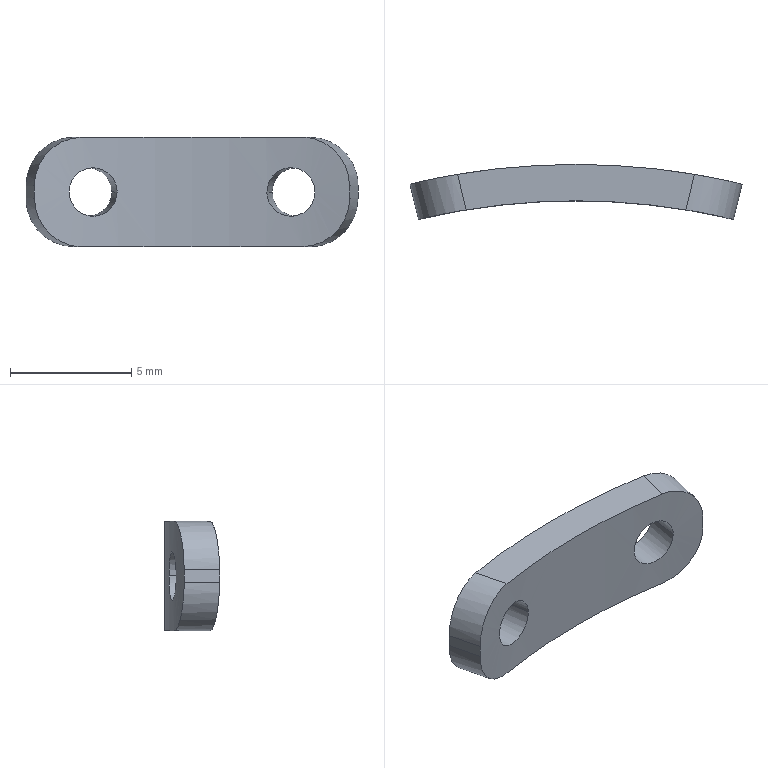Part | STEP file | 101000007769 | 1 solid | 14 faces | box 13.68 x 2.268 x 4.5 mm | volume 76.237 mm3 | cylinder 10 | plane 4 | commonest cylinder face diameters 2 x4 4 x4 55.6 x1 58.6 x1
STEP:
#1=CARTESIAN_POINT('',(5.284,28.82,0.));
#2=VERTEX_POINT('',#1);
#3=CARTESIAN_POINT('',(3.306,29.113,0.));
#4=VERTEX_POINT('',#3);
#5=CARTESIAN_POINT('',(5.284,28.82,0.));
#6=CARTESIAN_POINT('',(5.284,28.82,0.1258));
#7=CARTESIAN_POINT('',(5.265,28.823,0.2516));
#8=CARTESIAN_POINT('',(5.226,28.83,0.3686));
#9=CARTESIAN_POINT('',(5.12,28.849,0.5841));
#10=CARTESIAN_POINT('',(4.957,28.878,0.7588));
#11=CARTESIAN_POINT('',(4.861,28.894,0.8355));
#12=CARTESIAN_POINT('',(4.581,28.941,0.9925));
#13=CARTESIAN_POINT('',(4.255,28.99,1.029));
#14=CARTESIAN_POINT('',(4.056,29.019,1.));
#15=CARTESIAN_POINT('',(3.693,29.067,0.8498));
#16=CARTESIAN_POINT('',(3.438,29.098,0.5515));
#17=CARTESIAN_POINT('',(3.35,29.108,0.3772));
#18=CARTESIAN_POINT('',(3.306,29.113,0.1893));
#19=CARTESIAN_POINT('',(3.306,29.113,0.));
#20=B_SPLINE_CURVE_WITH_KNOTS('',5,(#5,#6,#7,#8,#9,#10,#11,#12,#13,#14,#15,#16,#17,#18,#19),.UNSPECIFIED.,.F.,.U.,(6,3,3,3,6),(0.,0.895,1.79,3.179,4.519),.UNSPECIFIED.);
#21=EDGE_CURVE('',#2,#4,#20,.T.);
#22=ORIENTED_EDGE('',*,*,#21,.F.);
#23=CARTESIAN_POINT('',(5.064,27.335,0.));
#24=VERTEX_POINT('',#23);
#25=CARTESIAN_POINT('',(0.9892,-0.1467,0.));
#26=DIRECTION('',(-0.1467,-0.9892,0.));
#27=VECTOR('',#26,1.);
#28=LINE('',#25,#27);
#29=EDGE_CURVE('',#2,#24,#28,.T.);
#30=ORIENTED_EDGE('',*,*,#29,.T.);
#31=CARTESIAN_POINT('',(3.086,27.628,0.));
#32=VERTEX_POINT('',#31);
#33=CARTESIAN_POINT('',(3.086,27.628,0.));
#34=CARTESIAN_POINT('',(3.086,27.628,0.07518));
#35=CARTESIAN_POINT('',(3.093,27.627,0.1502));
#36=CARTESIAN_POINT('',(3.106,27.626,0.222));
#37=CARTESIAN_POINT('',(3.146,27.621,0.3604));
#38=CARTESIAN_POINT('',(3.208,27.614,0.4897));
#39=CARTESIAN_POINT('',(3.246,27.61,0.5524));
#40=CARTESIAN_POINT('',(3.364,27.596,0.7128));
#41=CARTESIAN_POINT('',(3.519,27.577,0.84));
#42=CARTESIAN_POINT('',(3.625,27.563,0.902));
#43=CARTESIAN_POINT('',(3.85,27.533,0.9919));
#44=CARTESIAN_POINT('',(4.09,27.498,1.011));
#45=CARTESIAN_POINT('',(4.212,27.479,1.002));
#46=CARTESIAN_POINT('',(4.451,27.442,0.9461));
#47=CARTESIAN_POINT('',(4.661,27.407,0.8203));
#48=CARTESIAN_POINT('',(4.752,27.391,0.7439));
#49=CARTESIAN_POINT('',(4.909,27.363,0.569));
#50=CARTESIAN_POINT('',(5.01,27.345,0.3559));
#51=CARTESIAN_POINT('',(5.046,27.338,0.2414));
#52=CARTESIAN_POINT('',(5.064,27.335,0.1206));
#53=CARTESIAN_POINT('',(5.064,27.335,0.));
#54=B_SPLINE_CURVE_WITH_KNOTS('',5,(#33,#34,#35,#36,#37,#38,#39,#40,#41,#42,#43,#44,#45,#46,#47,#48,#49,#50,#51,#52,#53),.UNSPECIFIED.,.F.,.U.,(6,3,3,3,3,3,6),(0.,0.5314,1.063,1.943,2.823,3.679,4.536),.UNSPECIFIED.);
#55=EDGE_CURVE('',#32,#24,#54,.T.);
#56=ORIENTED_EDGE('',*,*,#55,.F.);
#57=CARTESIAN_POINT('',(-0.9892,0.1467,0.));
#58=DIRECTION('',(-0.1467,-0.9892,0.));
#59=VECTOR('',#58,1.);
#60=LINE('',#57,#59);
#61=EDGE_CURVE('',#4,#32,#60,.T.);
#62=ORIENTED_EDGE('',*,*,#61,.F.);
#63=EDGE_LOOP('',(#22,#30,#56,#62));
#64=FACE_OUTER_BOUND('',#63,.T.);
#65=CARTESIAN_POINT('',(0.,0.,0.));
#66=DIRECTION('',(-0.1467,-0.9892,0.));
#67=DIRECTION('',(0.9892,-0.1467,0.));
#68=AXIS2_PLACEMENT_3D('',#65,#66,#67);
#69=CYLINDRICAL_SURFACE('',#68,1.);
#70=ADVANCED_FACE('',(#64),#69,.F.);
#71=CARTESIAN_POINT('',(4.879,28.891,-2.25));
#72=VERTEX_POINT('',#71);
#73=CARTESIAN_POINT('',(-4.879,28.891,-2.25));
#74=VERTEX_POINT('',#73);
#75=CARTESIAN_POINT('',(0.,0.,-2.25));
#76=DIRECTION('',(0.,0.,-1.));
#77=AXIS2_PLACEMENT_3D('',#75,#76,$);
#78=CIRCLE('',#77,29.3);
#79=EDGE_CURVE('',#72,#74,#78,.F.);
#80=ORIENTED_EDGE('',*,*,#79,.T.);
#81=CARTESIAN_POINT('',(-6.84,28.49,-0.25));
#82=VERTEX_POINT('',#81);
#83=CARTESIAN_POINT('',(-4.879,28.891,-2.25));
#84=CARTESIAN_POINT('',(-5.502,28.786,-2.249));
#85=CARTESIAN_POINT('',(-6.113,28.666,-2.007));
#86=CARTESIAN_POINT('',(-6.603,28.547,-1.504));
#87=CARTESIAN_POINT('',(-6.84,28.491,-0.8818));
#88=CARTESIAN_POINT('',(-6.84,28.49,-0.25));
#89=B_SPLINE_CURVE_WITH_KNOTS('',5,(#83,#84,#85,#86,#87,#88),.UNSPECIFIED.,.F.,.U.,(6,6),(0.,4.453),.UNSPECIFIED.);
#90=EDGE_CURVE('',#74,#82,#89,.T.);
#91=ORIENTED_EDGE('',*,*,#90,.T.);
#92=CARTESIAN_POINT('',(-6.84,28.49,0.25));
#93=VERTEX_POINT('',#92);
#94=CARTESIAN_POINT('',(-6.84,28.49,2.25));
#95=DIRECTION('',(0.,0.,-1.));
#96=VECTOR('',#95,1.);
#97=LINE('',#94,#96);
#98=EDGE_CURVE('',#93,#82,#97,.T.);
#99=ORIENTED_EDGE('',*,*,#98,.F.);
#100=CARTESIAN_POINT('',(-4.879,28.891,2.25));
#101=VERTEX_POINT('',#100);
#102=CARTESIAN_POINT('',(-6.84,28.49,0.25));
#103=CARTESIAN_POINT('',(-6.839,28.491,0.8818));
#104=CARTESIAN_POINT('',(-6.602,28.547,1.504));
#105=CARTESIAN_POINT('',(-6.113,28.666,2.007));
#106=CARTESIAN_POINT('',(-5.502,28.786,2.25));
#107=CARTESIAN_POINT('',(-4.879,28.891,2.25));
#108=B_SPLINE_CURVE_WITH_KNOTS('',5,(#102,#103,#104,#105,#106,#107),.UNSPECIFIED.,.F.,.U.,(6,6),(0.,4.453),.UNSPECIFIED.);
#109=EDGE_CURVE('',#93,#101,#108,.T.);
#110=ORIENTED_EDGE('',*,*,#109,.T.);
#111=CARTESIAN_POINT('',(4.879,28.891,2.25));
#112=VERTEX_POINT('',#111);
#113=CARTESIAN_POINT('',(0.,0.,2.25));
#114=DIRECTION('',(0.,0.,-1.));
#115=AXIS2_PLACEMENT_3D('',#113,#114,$);
#116=CIRCLE('',#115,29.3);
#117=EDGE_CURVE('',#112,#101,#116,.F.);
#118=ORIENTED_EDGE('',*,*,#117,.F.);
#119=CARTESIAN_POINT('',(6.84,28.49,0.25));
#120=VERTEX_POINT('',#119);
#121=CARTESIAN_POINT('',(4.879,28.891,2.25));
#122=CARTESIAN_POINT('',(5.502,28.786,2.249));
#123=CARTESIAN_POINT('',(6.113,28.666,2.007));
#124=CARTESIAN_POINT('',(6.603,28.547,1.504));
#125=CARTESIAN_POINT('',(6.84,28.491,0.8818));
#126=CARTESIAN_POINT('',(6.84,28.49,0.25));
#127=B_SPLINE_CURVE_WITH_KNOTS('',5,(#121,#122,#123,#124,#125,#126),.UNSPECIFIED.,.F.,.U.,(6,6),(0.,4.453),.UNSPECIFIED.);
#128=EDGE_CURVE('',#112,#120,#127,.T.);
#129=ORIENTED_EDGE('',*,*,#128,.T.);
#130=CARTESIAN_POINT('',(6.84,28.49,-0.25));
#131=VERTEX_POINT('',#130);
#132=CARTESIAN_POINT('',(6.84,28.49,2.25));
#133=DIRECTION('',(0.,0.,-1.));
#134=VECTOR('',#133,1.);
#135=LINE('',#132,#134);
#136=EDGE_CURVE('',#120,#131,#135,.T.);
#137=ORIENTED_EDGE('',*,*,#136,.T.);
#138=CARTESIAN_POINT('',(6.84,28.49,-0.25));
#139=CARTESIAN_POINT('',(6.839,28.491,-0.8818));
#140=CARTESIAN_POINT('',(6.602,28.547,-1.504));
#141=CARTESIAN_POINT('',(6.113,28.666,-2.007));
#142=CARTESIAN_POINT('',(5.502,28.786,-2.25));
#143=CARTESIAN_POINT('',(4.879,28.891,-2.25));
#144=B_SPLINE_CURVE_WITH_KNOTS('',5,(#138,#139,#140,#141,#142,#143),.UNSPECIFIED.,.F.,.U.,(6,6),(0.,4.453),.UNSPECIFIED.);
#145=EDGE_CURVE('',#131,#72,#144,.T.);
#146=ORIENTED_EDGE('',*,*,#145,.T.);
#147=EDGE_LOOP('',(#80,#91,#99,#110,#118,#129,#137,#146));
#148=FACE_OUTER_BOUND('',#147,.T.);
#149=CARTESIAN_POINT('',(-3.306,29.113,0.));
#150=VERTEX_POINT('',#149);
#151=CARTESIAN_POINT('',(-5.284,28.82,0.));
#152=VERTEX_POINT('',#151);
#153=CARTESIAN_POINT('',(-3.306,29.113,0.));
#154=CARTESIAN_POINT('',(-3.306,29.113,0.2944));
#155=CARTESIAN_POINT('',(-3.414,29.101,0.586));
#156=CARTESIAN_POINT('',(-3.627,29.077,0.8257));
#157=CARTESIAN_POINT('',(-4.089,29.016,1.055));
#158=CARTESIAN_POINT('',(-4.582,28.941,0.9885));
#159=CARTESIAN_POINT('',(-4.77,28.91,0.9118));
#160=CARTESIAN_POINT('',(-5.044,28.863,0.7077));
#161=CARTESIAN_POINT('',(-5.212,28.833,0.4134));
#162=CARTESIAN_POINT('',(-5.26,28.824,0.2797));
#163=CARTESIAN_POINT('',(-5.284,28.82,0.1397));
#164=CARTESIAN_POINT('',(-5.284,28.82,0.));
#165=B_SPLINE_CURVE_WITH_KNOTS('',5,(#153,#154,#155,#156,#157,#158,#159,#160,#161,#162,#163,#164),.UNSPECIFIED.,.F.,.U.,(6,3,3,6),(0.,2.081,3.465,4.458),.UNSPECIFIED.);
#166=EDGE_CURVE('',#150,#152,#165,.T.);
#167=ORIENTED_EDGE('',*,*,#166,.T.);
#168=CARTESIAN_POINT('',(-5.284,28.82,0.));
#169=CARTESIAN_POINT('',(-5.284,28.82,-0.2936));
#170=CARTESIAN_POINT('',(-5.177,28.839,-0.5871));
#171=CARTESIAN_POINT('',(-4.966,28.878,-0.8262));
#172=CARTESIAN_POINT('',(-4.505,28.954,-1.055));
#173=CARTESIAN_POINT('',(-4.011,29.025,-0.988));
#174=CARTESIAN_POINT('',(-3.822,29.05,-0.911));
#175=CARTESIAN_POINT('',(-3.547,29.085,-0.7069));
#176=CARTESIAN_POINT('',(-3.38,29.105,-0.4129));
#177=CARTESIAN_POINT('',(-3.331,29.11,-0.2794));
#178=CARTESIAN_POINT('',(-3.306,29.113,-0.1401));
#179=CARTESIAN_POINT('',(-3.306,29.113,0.));
#180=B_SPLINE_CURVE_WITH_KNOTS('',5,(#168,#169,#170,#171,#172,#173,#174,#175,#176,#177,#178,#179),.UNSPECIFIED.,.F.,.U.,(6,3,3,6),(0.,2.088,3.475,4.466),.UNSPECIFIED.);
#181=EDGE_CURVE('',#152,#150,#180,.T.);
#182=ORIENTED_EDGE('',*,*,#181,.T.);
#183=EDGE_LOOP('',(#167,#182));
#184=FACE_BOUND('',#183,.T.);
#185=CARTESIAN_POINT('',(3.306,29.113,0.));
#186=CARTESIAN_POINT('',(3.306,29.113,-0.2944));
#187=CARTESIAN_POINT('',(3.414,29.101,-0.586));
#188=CARTESIAN_POINT('',(3.627,29.077,-0.8257));
#189=CARTESIAN_POINT('',(4.089,29.016,-1.055));
#190=CARTESIAN_POINT('',(4.582,28.941,-0.9885));
#191=CARTESIAN_POINT('',(4.77,28.91,-0.9118));
#192=CARTESIAN_POINT('',(5.044,28.863,-0.7077));
#193=CARTESIAN_POINT('',(5.212,28.833,-0.4134));
#194=CARTESIAN_POINT('',(5.26,28.824,-0.2797));
#195=CARTESIAN_POINT('',(5.284,28.82,-0.1397));
#196=CARTESIAN_POINT('',(5.284,28.82,0.));
#197=B_SPLINE_CURVE_WITH_KNOTS('',5,(#185,#186,#187,#188,#189,#190,#191,#192,#193,#194,#195,#196),.UNSPECIFIED.,.F.,.U.,(6,3,3,6),(0.,2.081,3.465,4.458),.UNSPECIFIED.);
#198=EDGE_CURVE('',#4,#2,#197,.T.);
#199=ORIENTED_EDGE('',*,*,#198,.T.);
#200=ORIENTED_EDGE('',*,*,#21,.T.);
#201=EDGE_LOOP('',(#199,#200));
#202=FACE_BOUND('',#201,.T.);
#203=CARTESIAN_POINT('',(0.,0.,2.25));
#204=DIRECTION('',(0.,0.,-1.));
#205=DIRECTION('',(-1.,0.,0.));
#206=AXIS2_PLACEMENT_3D('',#203,#204,#205);
#207=CYLINDRICAL_SURFACE('',#206,29.3);
#208=ADVANCED_FACE('',(#148,#184,#202),#207,.T.);
#209=ORIENTED_EDGE('',*,*,#29,.F.);
#210=ORIENTED_EDGE('',*,*,#198,.F.);
#211=ORIENTED_EDGE('',*,*,#61,.T.);
#212=CARTESIAN_POINT('',(5.064,27.335,0.));
#213=CARTESIAN_POINT('',(5.064,27.335,-0.1259));
#214=CARTESIAN_POINT('',(5.044,27.339,-0.2517));
#215=CARTESIAN_POINT('',(5.006,27.346,-0.3687));
#216=CARTESIAN_POINT('',(4.9,27.365,-0.5841));
#217=CARTESIAN_POINT('',(4.737,27.394,-0.7588));
#218=CARTESIAN_POINT('',(4.642,27.41,-0.8354));
#219=CARTESIAN_POINT('',(4.361,27.457,-0.9925));
#220=CARTESIAN_POINT('',(4.035,27.507,-1.029));
#221=CARTESIAN_POINT('',(3.836,27.535,-1.));
#222=CARTESIAN_POINT('',(3.473,27.583,-0.8498));
#223=CARTESIAN_POINT('',(3.218,27.613,-0.5515));
#224=CARTESIAN_POINT('',(3.13,27.623,-0.3773));
#225=CARTESIAN_POINT('',(3.086,27.628,-0.1893));
#226=CARTESIAN_POINT('',(3.086,27.628,0.));
#227=B_SPLINE_CURVE_WITH_KNOTS('',5,(#212,#213,#214,#215,#216,#217,#218,#219,#220,#221,#222,#223,#224,#225,#226),.UNSPECIFIED.,.F.,.U.,(6,3,3,3,6),(0.,0.8953,1.791,3.18,4.519),.UNSPECIFIED.);
#228=EDGE_CURVE('',#24,#32,#227,.T.);
#229=ORIENTED_EDGE('',*,*,#228,.F.);
#230=EDGE_LOOP('',(#209,#210,#211,#229));
#231=FACE_OUTER_BOUND('',#230,.T.);
#232=CARTESIAN_POINT('',(0.,0.,0.));
#233=DIRECTION('',(-0.1467,-0.9892,0.));
#234=DIRECTION('',(-0.9892,0.1467,0.));
#235=AXIS2_PLACEMENT_3D('',#232,#233,#234);
#236=CYLINDRICAL_SURFACE('',#235,1.);
#237=ADVANCED_FACE('',(#231),#236,.F.);
#238=CARTESIAN_POINT('',(-6.49,27.032,0.25));
#239=VERTEX_POINT('',#238);
#240=CARTESIAN_POINT('',(-6.49,27.032,-0.25));
#241=VERTEX_POINT('',#240);
#242=CARTESIAN_POINT('',(-6.49,27.032,2.25));
#243=DIRECTION('',(0.,0.,-1.));
#244=VECTOR('',#243,1.);
#245=LINE('',#242,#244);
#246=EDGE_CURVE('',#239,#241,#245,.T.);
#247=ORIENTED_EDGE('',*,*,#246,.T.);
#248=CARTESIAN_POINT('',(-4.528,27.429,-2.25));
#249=VERTEX_POINT('',#248);
#250=CARTESIAN_POINT('',(-6.49,27.032,-0.25));
#251=CARTESIAN_POINT('',(-6.489,27.032,-0.8818));
#252=CARTESIAN_POINT('',(-6.252,27.089,-1.504));
#253=CARTESIAN_POINT('',(-5.763,27.207,-2.007));
#254=CARTESIAN_POINT('',(-5.152,27.326,-2.25));
#255=CARTESIAN_POINT('',(-4.528,27.429,-2.25));
#256=B_SPLINE_CURVE_WITH_KNOTS('',5,(#250,#251,#252,#253,#254,#255),.UNSPECIFIED.,.F.,.U.,(6,6),(0.,4.453),.UNSPECIFIED.);
#257=EDGE_CURVE('',#241,#249,#256,.T.);
#258=ORIENTED_EDGE('',*,*,#257,.T.);
#259=CARTESIAN_POINT('',(4.528,27.429,-2.25));
#260=VERTEX_POINT('',#259);
#261=CARTESIAN_POINT('',(0.,0.,-2.25));
#262=DIRECTION('',(0.,0.,-1.));
#263=AXIS2_PLACEMENT_3D('',#261,#262,$);
#264=CIRCLE('',#263,27.8);
#265=EDGE_CURVE('',#249,#260,#264,.T.);
#266=ORIENTED_EDGE('',*,*,#265,.T.);
#267=CARTESIAN_POINT('',(6.49,27.032,-0.25));
#268=VERTEX_POINT('',#267);
#269=CARTESIAN_POINT('',(4.528,27.429,-2.25));
#270=CARTESIAN_POINT('',(5.152,27.326,-2.249));
#271=CARTESIAN_POINT('',(5.763,27.207,-2.007));
#272=CARTESIAN_POINT('',(6.253,27.089,-1.504));
#273=CARTESIAN_POINT('',(6.489,27.032,-0.8818));
#274=CARTESIAN_POINT('',(6.49,27.032,-0.25));
#275=B_SPLINE_CURVE_WITH_KNOTS('',5,(#269,#270,#271,#272,#273,#274),.UNSPECIFIED.,.F.,.U.,(6,6),(0.,4.453),.UNSPECIFIED.);
#276=EDGE_CURVE('',#260,#268,#275,.T.);
#277=ORIENTED_EDGE('',*,*,#276,.T.);
#278=CARTESIAN_POINT('',(6.49,27.032,0.25));
#279=VERTEX_POINT('',#278);
#280=CARTESIAN_POINT('',(6.49,27.032,2.25));
#281=DIRECTION('',(0.,0.,-1.));
#282=VECTOR('',#281,1.);
#283=LINE('',#280,#282);
#284=EDGE_CURVE('',#279,#268,#283,.T.);
#285=ORIENTED_EDGE('',*,*,#284,.F.);
#286=CARTESIAN_POINT('',(4.528,27.429,2.25));
#287=VERTEX_POINT('',#286);
#288=CARTESIAN_POINT('',(6.49,27.032,0.25));
#289=CARTESIAN_POINT('',(6.489,27.032,0.8818));
#290=CARTESIAN_POINT('',(6.252,27.089,1.504));
#291=CARTESIAN_POINT('',(5.763,27.207,2.007));
#292=CARTESIAN_POINT('',(5.152,27.326,2.25));
#293=CARTESIAN_POINT('',(4.528,27.429,2.25));
#294=B_SPLINE_CURVE_WITH_KNOTS('',5,(#288,#289,#290,#291,#292,#293),.UNSPECIFIED.,.F.,.U.,(6,6),(0.,4.453),.UNSPECIFIED.);
#295=EDGE_CURVE('',#279,#287,#294,.T.);
#296=ORIENTED_EDGE('',*,*,#295,.T.);
#297=CARTESIAN_POINT('',(-4.528,27.429,2.25));
#298=VERTEX_POINT('',#297);
#299=CARTESIAN_POINT('',(0.,0.,2.25));
#300=DIRECTION('',(0.,0.,-1.));
#301=AXIS2_PLACEMENT_3D('',#299,#300,$);
#302=CIRCLE('',#301,27.8);
#303=EDGE_CURVE('',#298,#287,#302,.T.);
#304=ORIENTED_EDGE('',*,*,#303,.F.);
#305=CARTESIAN_POINT('',(-4.528,27.429,2.25));
#306=CARTESIAN_POINT('',(-5.152,27.326,2.249));
#307=CARTESIAN_POINT('',(-5.763,27.207,2.007));
#308=CARTESIAN_POINT('',(-6.253,27.089,1.504));
#309=CARTESIAN_POINT('',(-6.489,27.032,0.8818));
#310=CARTESIAN_POINT('',(-6.49,27.032,0.25));
#311=B_SPLINE_CURVE_WITH_KNOTS('',5,(#305,#306,#307,#308,#309,#310),.UNSPECIFIED.,.F.,.U.,(6,6),(0.,4.453),.UNSPECIFIED.);
#312=EDGE_CURVE('',#298,#239,#311,.T.);
#313=ORIENTED_EDGE('',*,*,#312,.T.);
#314=EDGE_LOOP('',(#247,#258,#266,#277,#285,#296,#304,#313));
#315=FACE_OUTER_BOUND('',#314,.T.);
#316=CARTESIAN_POINT('',(-3.086,27.628,0.));
#317=VERTEX_POINT('',#316);
#318=CARTESIAN_POINT('',(-5.064,27.335,0.));
#319=VERTEX_POINT('',#318);
#320=CARTESIAN_POINT('',(-3.086,27.628,0.));
#321=CARTESIAN_POINT('',(-3.085,27.628,-0.2944));
#322=CARTESIAN_POINT('',(-3.194,27.616,-0.586));
#323=CARTESIAN_POINT('',(-3.407,27.593,-0.8257));
#324=CARTESIAN_POINT('',(-3.869,27.532,-1.055));
#325=CARTESIAN_POINT('',(-4.362,27.457,-0.9885));
#326=CARTESIAN_POINT('',(-4.55,27.426,-0.9118));
#327=CARTESIAN_POINT('',(-4.824,27.379,-0.7077));
#328=CARTESIAN_POINT('',(-4.992,27.348,-0.4134));
#329=CARTESIAN_POINT('',(-5.04,27.339,-0.2797));
#330=CARTESIAN_POINT('',(-5.064,27.335,-0.1397));
#331=CARTESIAN_POINT('',(-5.064,27.335,0.));
#332=B_SPLINE_CURVE_WITH_KNOTS('',5,(#320,#321,#322,#323,#324,#325,#326,#327,#328,#329,#330,#331),.UNSPECIFIED.,.F.,.U.,(6,3,3,6),(0.,2.081,3.465,4.458),.UNSPECIFIED.);
#333=EDGE_CURVE('',#317,#319,#332,.T.);
#334=ORIENTED_EDGE('',*,*,#333,.T.);
#335=CARTESIAN_POINT('',(-5.064,27.335,0.));
#336=CARTESIAN_POINT('',(-5.064,27.335,0.2936));
#337=CARTESIAN_POINT('',(-4.957,27.355,0.5871));
#338=CARTESIAN_POINT('',(-4.746,27.394,0.8262));
#339=CARTESIAN_POINT('',(-4.285,27.471,1.055));
#340=CARTESIAN_POINT('',(-3.791,27.541,0.988));
#341=CARTESIAN_POINT('',(-3.602,27.566,0.911));
#342=CARTESIAN_POINT('',(-3.327,27.601,0.7069));
#343=CARTESIAN_POINT('',(-3.16,27.62,0.4129));
#344=CARTESIAN_POINT('',(-3.111,27.625,0.2795));
#345=CARTESIAN_POINT('',(-3.085,27.628,0.1401));
#346=CARTESIAN_POINT('',(-3.086,27.628,0.));
#347=B_SPLINE_CURVE_WITH_KNOTS('',5,(#335,#336,#337,#338,#339,#340,#341,#342,#343,#344,#345,#346),.UNSPECIFIED.,.F.,.U.,(6,3,3,6),(0.,2.088,3.475,4.466),.UNSPECIFIED.);
#348=EDGE_CURVE('',#319,#317,#347,.T.);
#349=ORIENTED_EDGE('',*,*,#348,.T.);
#350=EDGE_LOOP('',(#334,#349));
#351=FACE_BOUND('',#350,.T.);
#352=ORIENTED_EDGE('',*,*,#55,.T.);
#353=ORIENTED_EDGE('',*,*,#228,.T.);
#354=EDGE_LOOP('',(#352,#353));
#355=FACE_BOUND('',#354,.T.);
#356=CARTESIAN_POINT('',(0.,0.,2.25));
#357=DIRECTION('',(0.,0.,-1.));
#358=DIRECTION('',(-1.,0.,0.));
#359=AXIS2_PLACEMENT_3D('',#356,#357,#358);
#360=CYLINDRICAL_SURFACE('',#359,27.8);
#361=ADVANCED_FACE('',(#315,#351,#355),#360,.F.);
#362=ORIENTED_EDGE('',*,*,#265,.F.);
#363=CARTESIAN_POINT('',(-4.704,28.16,-2.25));
#364=DIRECTION('',(-0.2334,0.9724,0.));
#365=VECTOR('',#364,1.);
#366=LINE('',#363,#365);
#367=EDGE_CURVE('',#249,#74,#366,.T.);
#368=ORIENTED_EDGE('',*,*,#367,.T.);
#369=ORIENTED_EDGE('',*,*,#79,.F.);
#370=CARTESIAN_POINT('',(4.704,28.16,-2.25));
#371=DIRECTION('',(-0.2334,-0.9724,0.));
#372=VECTOR('',#371,1.);
#373=LINE('',#370,#372);
#374=EDGE_CURVE('',#72,#260,#373,.T.);
#375=ORIENTED_EDGE('',*,*,#374,.T.);
#376=EDGE_LOOP('',(#362,#368,#369,#375));
#377=FACE_OUTER_BOUND('',#376,.T.);
#378=CARTESIAN_POINT('',(0.,0.,-2.25));
#379=DIRECTION('',(0.,0.,1.));
#380=DIRECTION('',(1.,0.,0.));
#381=AXIS2_PLACEMENT_3D('',#378,#379,#380);
#382=PLANE('',#381);
#383=ADVANCED_FACE('',(#377),#382,.F.);
#384=ORIENTED_EDGE('',*,*,#90,.F.);
#385=ORIENTED_EDGE('',*,*,#367,.F.);
#386=ORIENTED_EDGE('',*,*,#257,.F.);
#387=CARTESIAN_POINT('',(-6.84,28.49,-0.25));
#388=DIRECTION('',(0.2334,-0.9724,0.));
#389=VECTOR('',#388,1.);
#390=LINE('',#387,#389);
#391=EDGE_CURVE('',#82,#241,#390,.T.);
#392=ORIENTED_EDGE('',*,*,#391,.F.);
#393=EDGE_LOOP('',(#384,#385,#386,#392));
#394=FACE_OUTER_BOUND('',#393,.T.);
#395=CARTESIAN_POINT('',(-4.895,28.957,-0.25));
#396=DIRECTION('',(0.2334,-0.9724,0.));
#397=DIRECTION('',(-0.9724,-0.2334,0.));
#398=AXIS2_PLACEMENT_3D('',#395,#396,#397);
#399=CYLINDRICAL_SURFACE('',#398,2.);
#400=ADVANCED_FACE('',(#394),#399,.T.);
#401=ORIENTED_EDGE('',*,*,#98,.T.);
#402=ORIENTED_EDGE('',*,*,#391,.T.);
#403=ORIENTED_EDGE('',*,*,#246,.F.);
#404=CARTESIAN_POINT('',(-6.665,27.761,0.25));
#405=DIRECTION('',(-0.2334,0.9724,0.));
#406=VECTOR('',#405,1.);
#407=LINE('',#404,#406);
#408=EDGE_CURVE('',#239,#93,#407,.T.);
#409=ORIENTED_EDGE('',*,*,#408,.T.);
#410=EDGE_LOOP('',(#401,#402,#403,#409));
#411=FACE_OUTER_BOUND('',#410,.T.);
#412=CARTESIAN_POINT('',(-6.84,28.49,2.25));
#413=DIRECTION('',(0.9724,0.2334,0.));
#414=DIRECTION('',(-0.2334,0.9724,0.));
#415=AXIS2_PLACEMENT_3D('',#412,#413,#414);
#416=PLANE('',#415);
#417=ADVANCED_FACE('',(#411),#416,.F.);
#418=ORIENTED_EDGE('',*,*,#109,.F.);
#419=ORIENTED_EDGE('',*,*,#408,.F.);
#420=ORIENTED_EDGE('',*,*,#312,.F.);
#421=CARTESIAN_POINT('',(1.945,0.4669,2.25));
#422=DIRECTION('',(-0.2334,0.9724,0.));
#423=VECTOR('',#422,1.);
#424=LINE('',#421,#423);
#425=EDGE_CURVE('',#101,#298,#424,.F.);
#426=ORIENTED_EDGE('',*,*,#425,.F.);
#427=EDGE_LOOP('',(#418,#419,#420,#426));
#428=FACE_OUTER_BOUND('',#427,.T.);
#429=CARTESIAN_POINT('',(1.945,0.4669,0.25));
#430=DIRECTION('',(-0.2334,0.9724,0.));
#431=DIRECTION('',(-0.9724,-0.2334,0.));
#432=AXIS2_PLACEMENT_3D('',#429,#430,#431);
#433=CYLINDRICAL_SURFACE('',#432,2.);
#434=ADVANCED_FACE('',(#428),#433,.T.);
#435=ORIENTED_EDGE('',*,*,#303,.T.);
#436=CARTESIAN_POINT('',(4.704,28.16,2.25));
#437=DIRECTION('',(0.2334,0.9724,0.));
#438=VECTOR('',#437,1.);
#439=LINE('',#436,#438);
#440=EDGE_CURVE('',#287,#112,#439,.T.);
#441=ORIENTED_EDGE('',*,*,#440,.T.);
#442=ORIENTED_EDGE('',*,*,#117,.T.);
#443=ORIENTED_EDGE('',*,*,#425,.T.);
#444=EDGE_LOOP('',(#435,#441,#442,#443));
#445=FACE_OUTER_BOUND('',#444,.T.);
#446=CARTESIAN_POINT('',(0.,0.,2.25));
#447=DIRECTION('',(0.,0.,1.));
#448=DIRECTION('',(1.,0.,0.));
#449=AXIS2_PLACEMENT_3D('',#446,#447,#448);
#450=PLANE('',#449);
#451=ADVANCED_FACE('',(#445),#450,.T.);
#452=ORIENTED_EDGE('',*,*,#295,.F.);
#453=CARTESIAN_POINT('',(0.,0.,0.25));
#454=DIRECTION('',(-0.2334,-0.9724,0.));
#455=VECTOR('',#454,1.);
#456=LINE('',#453,#455);
#457=EDGE_CURVE('',#120,#279,#456,.T.);
#458=ORIENTED_EDGE('',*,*,#457,.F.);
#459=ORIENTED_EDGE('',*,*,#128,.F.);
#460=ORIENTED_EDGE('',*,*,#440,.F.);
#461=EDGE_LOOP('',(#452,#458,#459,#460));
#462=FACE_OUTER_BOUND('',#461,.T.);
#463=CARTESIAN_POINT('',(-1.945,0.4669,0.25));
#464=DIRECTION('',(-0.2334,-0.9724,0.));
#465=DIRECTION('',(0.9724,-0.2334,0.));
#466=AXIS2_PLACEMENT_3D('',#463,#464,#465);
#467=CYLINDRICAL_SURFACE('',#466,2.);
#468=ADVANCED_FACE('',(#462),#467,.T.);
#469=ORIENTED_EDGE('',*,*,#284,.T.);
#470=CARTESIAN_POINT('',(6.665,27.761,-0.25));
#471=DIRECTION('',(0.2334,0.9724,0.));
#472=VECTOR('',#471,1.);
#473=LINE('',#470,#472);
#474=EDGE_CURVE('',#268,#131,#473,.T.);
#475=ORIENTED_EDGE('',*,*,#474,.T.);
#476=ORIENTED_EDGE('',*,*,#136,.F.);
#477=ORIENTED_EDGE('',*,*,#457,.T.);
#478=EDGE_LOOP('',(#469,#475,#476,#477));
#479=FACE_OUTER_BOUND('',#478,.T.);
#480=CARTESIAN_POINT('',(6.84,28.49,2.25));
#481=DIRECTION('',(-0.9724,0.2334,0.));
#482=DIRECTION('',(-0.2334,-0.9724,0.));
#483=AXIS2_PLACEMENT_3D('',#480,#481,#482);
#484=PLANE('',#483);
#485=ADVANCED_FACE('',(#479),#484,.F.);
#486=ORIENTED_EDGE('',*,*,#276,.F.);
#487=ORIENTED_EDGE('',*,*,#374,.F.);
#488=ORIENTED_EDGE('',*,*,#145,.F.);
#489=ORIENTED_EDGE('',*,*,#474,.F.);
#490=EDGE_LOOP('',(#486,#487,#488,#489));
#491=FACE_OUTER_BOUND('',#490,.T.);
#492=CARTESIAN_POINT('',(4.895,28.957,-0.25));
#493=DIRECTION('',(0.2334,0.9724,0.));
#494=DIRECTION('',(0.9724,-0.2334,0.));
#495=AXIS2_PLACEMENT_3D('',#492,#493,#494);
#496=CYLINDRICAL_SURFACE('',#495,2.);
#497=ADVANCED_FACE('',(#491),#496,.T.);
#498=CARTESIAN_POINT('',(-0.9892,-0.1467,0.));
#499=DIRECTION('',(0.1467,-0.9892,0.));
#500=VECTOR('',#499,1.);
#501=LINE('',#498,#500);
#502=EDGE_CURVE('',#152,#319,#501,.T.);
#503=ORIENTED_EDGE('',*,*,#502,.F.);
#504=ORIENTED_EDGE('',*,*,#166,.F.);
#505=CARTESIAN_POINT('',(0.9892,0.1467,0.));
#506=DIRECTION('',(0.1467,-0.9892,0.));
#507=VECTOR('',#506,1.);
#508=LINE('',#505,#507);
#509=EDGE_CURVE('',#150,#317,#508,.T.);
#510=ORIENTED_EDGE('',*,*,#509,.T.);
#511=ORIENTED_EDGE('',*,*,#348,.F.);
#512=EDGE_LOOP('',(#503,#504,#510,#511));
#513=FACE_OUTER_BOUND('',#512,.T.);
#514=CARTESIAN_POINT('',(0.,0.,0.));
#515=DIRECTION('',(0.1467,-0.9892,0.));
#516=DIRECTION('',(0.9892,0.1467,0.));
#517=AXIS2_PLACEMENT_3D('',#514,#515,#516);
#518=CYLINDRICAL_SURFACE('',#517,1.);
#519=ADVANCED_FACE('',(#513),#518,.F.);
#520=ORIENTED_EDGE('',*,*,#181,.F.);
#521=ORIENTED_EDGE('',*,*,#502,.T.);
#522=ORIENTED_EDGE('',*,*,#333,.F.);
#523=ORIENTED_EDGE('',*,*,#509,.F.);
#524=EDGE_LOOP('',(#520,#521,#522,#523));
#525=FACE_OUTER_BOUND('',#524,.T.);
#526=CARTESIAN_POINT('',(0.,0.,0.));
#527=DIRECTION('',(0.1467,-0.9892,0.));
#528=DIRECTION('',(-0.9892,-0.1467,0.));
#529=AXIS2_PLACEMENT_3D('',#526,#527,#528);
#530=CYLINDRICAL_SURFACE('',#529,1.);
#531=ADVANCED_FACE('',(#525),#530,.F.);
#532=CLOSED_SHELL('',(#70,#208,#237,#361,#383,#400,#417,#434,#451,#468,#485,#497,#519,#531));
#533=MANIFOLD_SOLID_BREP('',#532);
#534=(LENGTH_UNIT()NAMED_UNIT(*)SI_UNIT(.MILLI.,.METRE.));
#535=UNCERTAINTY_MEASURE_WITH_UNIT(LENGTH_MEASURE(0.005),#534,'','');
#536=(NAMED_UNIT(*)PLANE_ANGLE_UNIT()SI_UNIT($,.RADIAN.));
#537=(NAMED_UNIT(*)SI_UNIT($,.STERADIAN.)SOLID_ANGLE_UNIT());
#538=(GEOMETRIC_REPRESENTATION_CONTEXT(3)GLOBAL_UNCERTAINTY_ASSIGNED_CONTEXT((#535))GLOBAL_UNIT_ASSIGNED_CONTEXT((#534,#536,#537))REPRESENTATION_CONTEXT('',''));
#539=ADVANCED_BREP_SHAPE_REPRESENTATION('',(#533),#538);